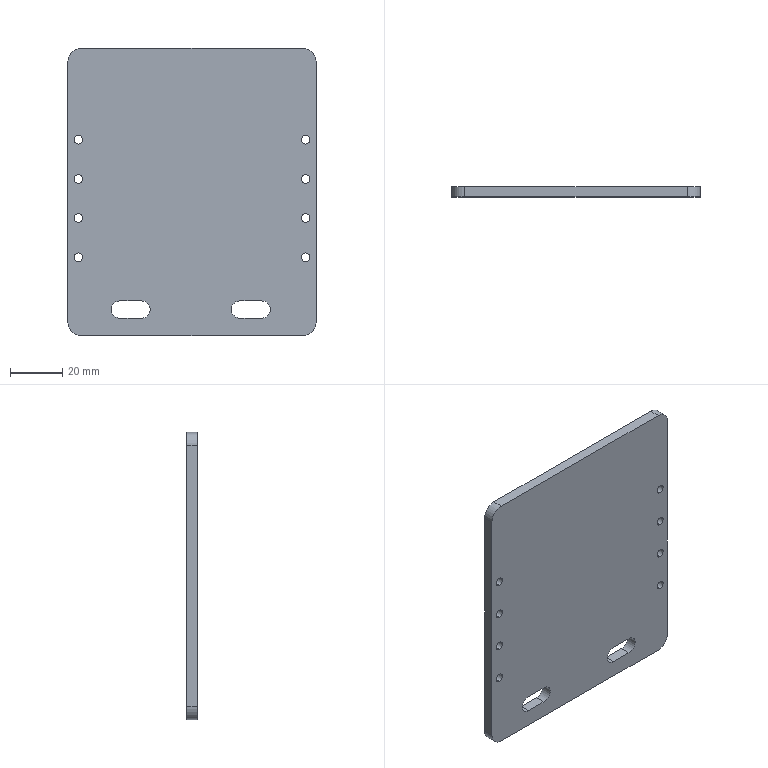Part | STEP file | 1 solid | 34 faces | box 95 x 4 x 110 mm | volume 40723 mm3 | cylinder 24 | plane 10 | commonest cylinder face diameters 3.3 x16 6.6 x4 10 x4